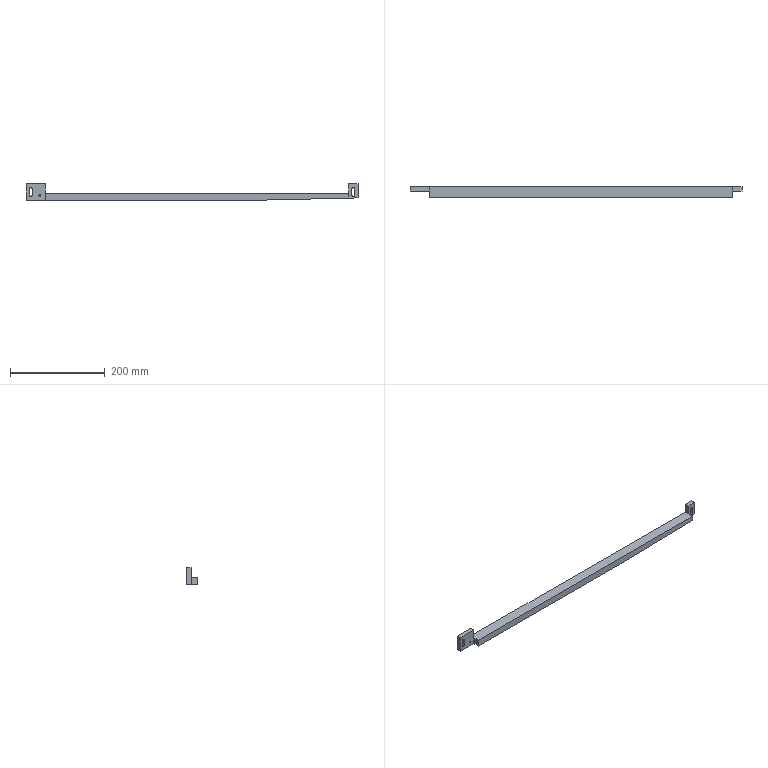Part | STEP file | PN_0013 | 1 solid | 31 faces | box 700 x 22 x 35 mm | volume 217020 mm3 | plane 19 | cylinder 10 | cone 2 | commonest cylinder face diameters 6.5 x6 3.3 x4